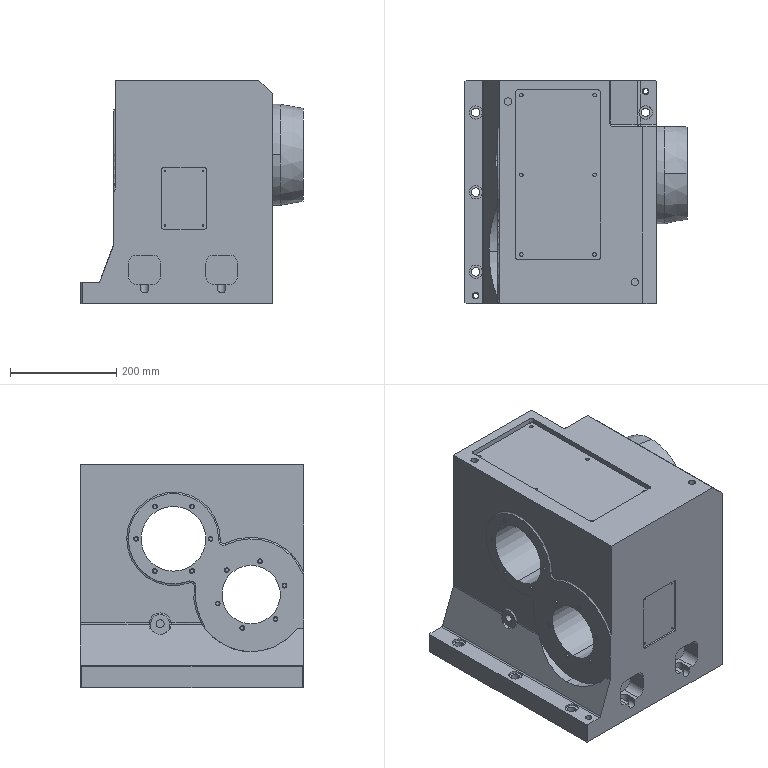Part | NX | features solid 2 | 1 solid | 326 faces | box 418 x 420 x 420 mm | volume 44013848 mm3 | cylinder 179 | plane 123 | torus 10 | spline 6 | cone 6 | sphere 2 | commonest cylinder face diameters 6.647 x36 16 x29 30 x28 9 x24 10 x19 2.459 x8